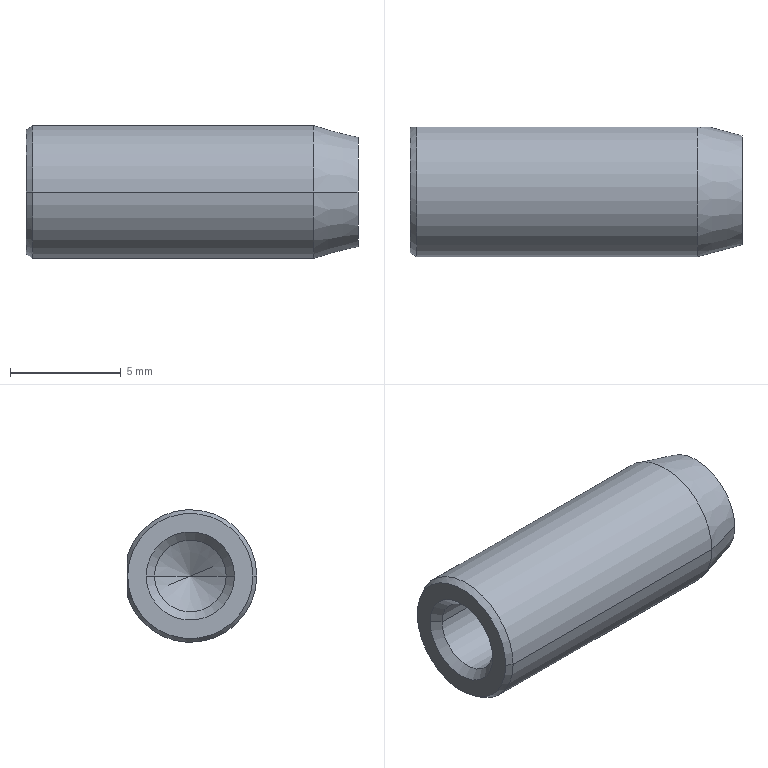Part | STEP file | MSTMS6-15-8 | 1 solid | 15 faces | box 15 x 5.85 x 6 mm | volume 330.192 mm3 | cone 8 | cylinder 4 | plane 3 | commonest cylinder face diameters 3.242 x2 6 x2
STEP:
#1=CARTESIAN_POINT('',(0.,0.,0.));
#2=DIRECTION('',(0.,0.,1.));
#3=DIRECTION('',(1.,0.,0.));
#4=AXIS2_PLACEMENT_3D('',#1,#2,#3);
#5=CARTESIAN_POINT('',(9.464,1.621,0.));
#6=VERTEX_POINT('',#5);
#7=CARTESIAN_POINT('',(9.464,-1.621,0.));
#8=VERTEX_POINT('',#7);
#9=CARTESIAN_POINT('',(9.464,0.,0.));
#10=DIRECTION('',(1.,0.,0.));
#11=DIRECTION('',(0.,-1.,0.));
#12=AXIS2_PLACEMENT_3D('',#9,#10,#11);
#13=CIRCLE('',#12,1.621);
#14=CARTESIAN_POINT('',(9.464,0.,0.));
#15=DIRECTION('',(-1.,0.,0.));
#16=DIRECTION('',(0.,1.,0.));
#17=AXIS2_PLACEMENT_3D('',#14,#15,#16);
#18=CONICAL_SURFACE('',#17,1.621,1.047);
#19=CARTESIAN_POINT('',(9.425,0.));
#20=DIRECTION('',(-1.,0.));
#21=VECTOR('',#20,1.);
#22=LINE('',#19,#21);
#23=(GEOMETRIC_REPRESENTATION_CONTEXT(2)PARAMETRIC_REPRESENTATION_CONTEXT()REPRESENTATION_CONTEXT('',''));
#24=DEFINITIONAL_REPRESENTATION('',(#22),#23);
#25=PCURVE('',#18,#24);
#26=CARTESIAN_POINT('',(10.4,0.,0.));
#27=DIRECTION('',(1.,0.,0.));
#28=DIRECTION('',(0.,-1.,0.));
#29=AXIS2_PLACEMENT_3D('',#26,#27,#28);
#30=CYLINDRICAL_SURFACE('',#29,1.621);
#31=CARTESIAN_POINT('',(0.,-0.9359));
#32=DIRECTION('',(1.,0.));
#33=VECTOR('',#32,1.);
#34=LINE('',#31,#33);
#35=(GEOMETRIC_REPRESENTATION_CONTEXT(2)PARAMETRIC_REPRESENTATION_CONTEXT()REPRESENTATION_CONTEXT('',''));
#36=DEFINITIONAL_REPRESENTATION('',(#34),#35);
#37=PCURVE('',#30,#36);
#38=SURFACE_CURVE('',#13,(#25,#37),.PCURVE_S1.);
#39=EDGE_CURVE('',#6,#8,#38,.T.);
#40=ORIENTED_EDGE('',*,*,#39,.T.);
#41=CARTESIAN_POINT('',(10.4,0.,0.));
#42=VERTEX_POINT('',#41);
#43=CARTESIAN_POINT('',(9.464,-1.621,0.));
#44=DIRECTION('',(-0.5,-0.866,0.));
#45=VECTOR('',#44,1.);
#46=LINE('',#43,#45);
#47=CARTESIAN_POINT('',(3.142,0.));
#48=DIRECTION('',(0.,1.));
#49=VECTOR('',#48,1.);
#50=LINE('',#47,#49);
#51=(GEOMETRIC_REPRESENTATION_CONTEXT(2)PARAMETRIC_REPRESENTATION_CONTEXT()REPRESENTATION_CONTEXT('',''));
#52=DEFINITIONAL_REPRESENTATION('',(#50),#51);
#53=PCURVE('',#18,#52);
#54=CARTESIAN_POINT('',(9.464,0.,0.));
#55=DIRECTION('',(-1.,0.,0.));
#56=DIRECTION('',(0.,1.,0.));
#57=AXIS2_PLACEMENT_3D('',#54,#55,#56);
#58=CONICAL_SURFACE('',#57,1.621,1.047);
#59=CARTESIAN_POINT('',(3.142,0.));
#60=DIRECTION('',(0.,1.));
#61=VECTOR('',#60,1.);
#62=LINE('',#59,#61);
#63=(GEOMETRIC_REPRESENTATION_CONTEXT(2)PARAMETRIC_REPRESENTATION_CONTEXT()REPRESENTATION_CONTEXT('',''));
#64=DEFINITIONAL_REPRESENTATION('',(#62),#63);
#65=PCURVE('',#58,#64);
#66=SURFACE_CURVE('',#46,(#53,#65),.PCURVE_S1.);
#67=EDGE_CURVE('',#42,#8,#66,.T.);
#68=ORIENTED_EDGE('',*,*,#67,.F.);
#69=CARTESIAN_POINT('',(9.464,1.621,0.));
#70=DIRECTION('',(-0.5,0.866,0.));
#71=VECTOR('',#70,1.);
#72=LINE('',#69,#71);
#73=CARTESIAN_POINT('',(6.283,0.));
#74=DIRECTION('',(0.,1.));
#75=VECTOR('',#74,1.);
#76=LINE('',#73,#75);
#77=(GEOMETRIC_REPRESENTATION_CONTEXT(2)PARAMETRIC_REPRESENTATION_CONTEXT()REPRESENTATION_CONTEXT('',''));
#78=DEFINITIONAL_REPRESENTATION('',(#76),#77);
#79=PCURVE('',#18,#78);
#80=CARTESIAN_POINT('',(0.,0.));
#81=DIRECTION('',(0.,1.));
#82=VECTOR('',#81,1.);
#83=LINE('',#80,#82);
#84=(GEOMETRIC_REPRESENTATION_CONTEXT(2)PARAMETRIC_REPRESENTATION_CONTEXT()REPRESENTATION_CONTEXT('',''));
#85=DEFINITIONAL_REPRESENTATION('',(#83),#84);
#86=PCURVE('',#58,#85);
#87=SURFACE_CURVE('',#72,(#79,#86),.PCURVE_S1.);
#88=EDGE_CURVE('',#42,#6,#87,.T.);
#89=ORIENTED_EDGE('',*,*,#88,.T.);
#90=EDGE_LOOP('',(#40,#68,#89));
#91=FACE_BOUND('',#90,.F.);
#92=ADVANCED_FACE('',(#91),#18,.F.);
#93=CARTESIAN_POINT('',(0.379,-1.621,0.));
#94=VERTEX_POINT('',#93);
#95=CARTESIAN_POINT('',(10.4,-1.621,0.));
#96=DIRECTION('',(1.,0.,0.));
#97=VECTOR('',#96,1.);
#98=LINE('',#95,#97);
#99=CARTESIAN_POINT('',(6.283,0.));
#100=DIRECTION('',(0.,1.));
#101=VECTOR('',#100,1.);
#102=LINE('',#99,#101);
#103=(GEOMETRIC_REPRESENTATION_CONTEXT(2)PARAMETRIC_REPRESENTATION_CONTEXT()REPRESENTATION_CONTEXT('',''));
#104=DEFINITIONAL_REPRESENTATION('',(#102),#103);
#105=PCURVE('',#30,#104);
#106=CARTESIAN_POINT('',(10.4,0.,0.));
#107=DIRECTION('',(1.,0.,0.));
#108=DIRECTION('',(0.,-1.,0.));
#109=AXIS2_PLACEMENT_3D('',#106,#107,#108);
#110=CYLINDRICAL_SURFACE('',#109,1.621);
#111=CARTESIAN_POINT('',(0.,0.));
#112=DIRECTION('',(0.,1.));
#113=VECTOR('',#112,1.);
#114=LINE('',#111,#113);
#115=(GEOMETRIC_REPRESENTATION_CONTEXT(2)PARAMETRIC_REPRESENTATION_CONTEXT()REPRESENTATION_CONTEXT('',''));
#116=DEFINITIONAL_REPRESENTATION('',(#114),#115);
#117=PCURVE('',#110,#116);
#118=SURFACE_CURVE('',#98,(#105,#117),.PCURVE_S1.);
#119=EDGE_CURVE('',#94,#8,#118,.T.);
#120=ORIENTED_EDGE('',*,*,#119,.T.);
#121=ORIENTED_EDGE('',*,*,#39,.F.);
#122=CARTESIAN_POINT('',(0.379,1.621,0.));
#123=VERTEX_POINT('',#122);
#124=CARTESIAN_POINT('',(10.4,1.621,0.));
#125=DIRECTION('',(1.,0.,0.));
#126=VECTOR('',#125,1.);
#127=LINE('',#124,#126);
#128=CARTESIAN_POINT('',(3.142,0.));
#129=DIRECTION('',(0.,1.));
#130=VECTOR('',#129,1.);
#131=LINE('',#128,#130);
#132=(GEOMETRIC_REPRESENTATION_CONTEXT(2)PARAMETRIC_REPRESENTATION_CONTEXT()REPRESENTATION_CONTEXT('',''));
#133=DEFINITIONAL_REPRESENTATION('',(#131),#132);
#134=PCURVE('',#30,#133);
#135=CARTESIAN_POINT('',(3.142,0.));
#136=DIRECTION('',(0.,1.));
#137=VECTOR('',#136,1.);
#138=LINE('',#135,#137);
#139=(GEOMETRIC_REPRESENTATION_CONTEXT(2)PARAMETRIC_REPRESENTATION_CONTEXT()REPRESENTATION_CONTEXT('',''));
#140=DEFINITIONAL_REPRESENTATION('',(#138),#139);
#141=PCURVE('',#110,#140);
#142=SURFACE_CURVE('',#127,(#134,#141),.PCURVE_S1.);
#143=EDGE_CURVE('',#123,#6,#142,.T.);
#144=ORIENTED_EDGE('',*,*,#143,.F.);
#145=CARTESIAN_POINT('',(0.379,0.,0.));
#146=DIRECTION('',(1.,0.,0.));
#147=DIRECTION('',(0.,-1.,0.));
#148=AXIS2_PLACEMENT_3D('',#145,#146,#147);
#149=CIRCLE('',#148,1.621);
#150=CARTESIAN_POINT('',(0.,-10.021));
#151=DIRECTION('',(1.,0.));
#152=VECTOR('',#151,1.);
#153=LINE('',#150,#152);
#154=(GEOMETRIC_REPRESENTATION_CONTEXT(2)PARAMETRIC_REPRESENTATION_CONTEXT()REPRESENTATION_CONTEXT('',''));
#155=DEFINITIONAL_REPRESENTATION('',(#153),#154);
#156=PCURVE('',#30,#155);
#157=CARTESIAN_POINT('',(0.,0.,0.));
#158=DIRECTION('',(-1.,0.,0.));
#159=DIRECTION('',(0.,1.,0.));
#160=AXIS2_PLACEMENT_3D('',#157,#158,#159);
#161=CONICAL_SURFACE('',#160,2.,0.7854);
#162=CARTESIAN_POINT('',(9.425,-0.379));
#163=DIRECTION('',(-1.,0.));
#164=VECTOR('',#163,1.);
#165=LINE('',#162,#164);
#166=(GEOMETRIC_REPRESENTATION_CONTEXT(2)PARAMETRIC_REPRESENTATION_CONTEXT()REPRESENTATION_CONTEXT('',''));
#167=DEFINITIONAL_REPRESENTATION('',(#165),#166);
#168=PCURVE('',#161,#167);
#169=SURFACE_CURVE('',#149,(#156,#168),.PCURVE_S1.);
#170=EDGE_CURVE('',#123,#94,#169,.T.);
#171=ORIENTED_EDGE('',*,*,#170,.T.);
#172=EDGE_LOOP('',(#120,#121,#144,#171));
#173=FACE_BOUND('',#172,.F.);
#174=ADVANCED_FACE('',(#173),#30,.F.);
#175=CARTESIAN_POINT('',(0.,2.,0.));
#176=VERTEX_POINT('',#175);
#177=CARTESIAN_POINT('',(0.,2.,0.));
#178=DIRECTION('',(-0.7071,0.7071,0.));
#179=VECTOR('',#178,1.);
#180=LINE('',#177,#179);
#181=CARTESIAN_POINT('',(6.283,0.));
#182=DIRECTION('',(0.,1.));
#183=VECTOR('',#182,1.);
#184=LINE('',#181,#183);
#185=(GEOMETRIC_REPRESENTATION_CONTEXT(2)PARAMETRIC_REPRESENTATION_CONTEXT()REPRESENTATION_CONTEXT('',''));
#186=DEFINITIONAL_REPRESENTATION('',(#184),#185);
#187=PCURVE('',#161,#186);
#188=CARTESIAN_POINT('',(0.,0.,0.));
#189=DIRECTION('',(-1.,0.,0.));
#190=DIRECTION('',(0.,1.,0.));
#191=AXIS2_PLACEMENT_3D('',#188,#189,#190);
#192=CONICAL_SURFACE('',#191,2.,0.7854);
#193=CARTESIAN_POINT('',(0.,0.));
#194=DIRECTION('',(0.,1.));
#195=VECTOR('',#194,1.);
#196=LINE('',#193,#195);
#197=(GEOMETRIC_REPRESENTATION_CONTEXT(2)PARAMETRIC_REPRESENTATION_CONTEXT()REPRESENTATION_CONTEXT('',''));
#198=DEFINITIONAL_REPRESENTATION('',(#196),#197);
#199=PCURVE('',#192,#198);
#200=SURFACE_CURVE('',#180,(#187,#199),.PCURVE_S1.);
#201=EDGE_CURVE('',#123,#176,#200,.T.);
#202=ORIENTED_EDGE('',*,*,#201,.T.);
#203=CARTESIAN_POINT('',(0.,-2.,0.));
#204=VERTEX_POINT('',#203);
#205=CARTESIAN_POINT('',(0.,0.,0.));
#206=DIRECTION('',(1.,0.,0.));
#207=DIRECTION('',(0.,-1.,0.));
#208=AXIS2_PLACEMENT_3D('',#205,#206,#207);
#209=CIRCLE('',#208,2.);
#210=CARTESIAN_POINT('',(9.425,0.));
#211=DIRECTION('',(-1.,0.));
#212=VECTOR('',#211,1.);
#213=LINE('',#210,#212);
#214=(GEOMETRIC_REPRESENTATION_CONTEXT(2)PARAMETRIC_REPRESENTATION_CONTEXT()REPRESENTATION_CONTEXT('',''));
#215=DEFINITIONAL_REPRESENTATION('',(#213),#214);
#216=PCURVE('',#161,#215);
#217=CARTESIAN_POINT('',(0.,0.,0.));
#218=DIRECTION('',(1.,0.,0.));
#219=DIRECTION('',(0.,-1.,0.));
#220=AXIS2_PLACEMENT_3D('',#217,#218,#219);
#221=PLANE('',#220);
#222=CARTESIAN_POINT('',(0.,0.));
#223=DIRECTION('',(1.,0.));
#224=AXIS2_PLACEMENT_2D('',#222,#223);
#225=CIRCLE('',#224,2.);
#226=(GEOMETRIC_REPRESENTATION_CONTEXT(2)PARAMETRIC_REPRESENTATION_CONTEXT()REPRESENTATION_CONTEXT('',''));
#227=DEFINITIONAL_REPRESENTATION('',(#225),#226);
#228=PCURVE('',#221,#227);
#229=SURFACE_CURVE('',#209,(#216,#228),.PCURVE_S1.);
#230=EDGE_CURVE('',#176,#204,#229,.T.);
#231=ORIENTED_EDGE('',*,*,#230,.T.);
#232=CARTESIAN_POINT('',(0.,-2.,0.));
#233=DIRECTION('',(-0.7071,-0.7071,0.));
#234=VECTOR('',#233,1.);
#235=LINE('',#232,#234);
#236=CARTESIAN_POINT('',(3.142,0.));
#237=DIRECTION('',(0.,1.));
#238=VECTOR('',#237,1.);
#239=LINE('',#236,#238);
#240=(GEOMETRIC_REPRESENTATION_CONTEXT(2)PARAMETRIC_REPRESENTATION_CONTEXT()REPRESENTATION_CONTEXT('',''));
#241=DEFINITIONAL_REPRESENTATION('',(#239),#240);
#242=PCURVE('',#161,#241);
#243=CARTESIAN_POINT('',(3.142,0.));
#244=DIRECTION('',(0.,1.));
#245=VECTOR('',#244,1.);
#246=LINE('',#243,#245);
#247=(GEOMETRIC_REPRESENTATION_CONTEXT(2)PARAMETRIC_REPRESENTATION_CONTEXT()REPRESENTATION_CONTEXT('',''));
#248=DEFINITIONAL_REPRESENTATION('',(#246),#247);
#249=PCURVE('',#192,#248);
#250=SURFACE_CURVE('',#235,(#242,#249),.PCURVE_S1.);
#251=EDGE_CURVE('',#94,#204,#250,.T.);
#252=ORIENTED_EDGE('',*,*,#251,.F.);
#253=ORIENTED_EDGE('',*,*,#170,.F.);
#254=EDGE_LOOP('',(#202,#231,#252,#253));
#255=FACE_BOUND('',#254,.F.);
#256=ADVANCED_FACE('',(#255),#161,.F.);
#257=CARTESIAN_POINT('',(15.,-2.464,0.));
#258=VERTEX_POINT('',#257);
#259=CARTESIAN_POINT('',(15.,2.464,0.));
#260=VERTEX_POINT('',#259);
#261=CARTESIAN_POINT('',(15.,0.,0.));
#262=DIRECTION('',(1.,0.,0.));
#263=DIRECTION('',(0.,-1.,0.));
#264=AXIS2_PLACEMENT_3D('',#261,#262,#263);
#265=CIRCLE('',#264,2.464);
#266=CARTESIAN_POINT('',(13.,0.,0.));
#267=DIRECTION('',(-1.,0.,0.));
#268=DIRECTION('',(0.,1.,0.));
#269=AXIS2_PLACEMENT_3D('',#266,#267,#268);
#270=CONICAL_SURFACE('',#269,3.,0.2618);
#271=CARTESIAN_POINT('',(3.142,-2.));
#272=DIRECTION('',(-1.,0.));
#273=VECTOR('',#272,1.);
#274=LINE('',#271,#273);
#275=(GEOMETRIC_REPRESENTATION_CONTEXT(2)PARAMETRIC_REPRESENTATION_CONTEXT()REPRESENTATION_CONTEXT('',''));
#276=DEFINITIONAL_REPRESENTATION('',(#274),#275);
#277=PCURVE('',#270,#276);
#278=CARTESIAN_POINT('',(15.,0.,-2.464));
#279=DIRECTION('',(-1.,0.,0.));
#280=DIRECTION('',(0.,1.,0.));
#281=AXIS2_PLACEMENT_3D('',#278,#279,#280);
#282=PLANE('',#281);
#283=CARTESIAN_POINT('',(-2.464,-2.464));
#284=CARTESIAN_POINT('',(-2.464,1.804));
#285=CARTESIAN_POINT('',(1.232,-0.3301));
#286=CARTESIAN_POINT('',(4.928,-2.464));
#287=CARTESIAN_POINT('',(1.232,-4.598));
#288=CARTESIAN_POINT('',(-2.464,-6.732));
#289=CARTESIAN_POINT('',(-2.464,-2.464));
#290=(BOUNDED_CURVE()B_SPLINE_CURVE(2,(#283,#284,#285,#286,#287,#288,#289),.UNSPECIFIED.,.T.,.F.)B_SPLINE_CURVE_WITH_KNOTS((1,2,2,2,2,1),(-2.094,0.,2.094,4.189,6.283,8.378),.UNSPECIFIED.)CURVE()GEOMETRIC_REPRESENTATION_ITEM()RATIONAL_B_SPLINE_CURVE((1.,0.5,1.,0.5,1.,0.5,1.))REPRESENTATION_ITEM(''));
#291=(GEOMETRIC_REPRESENTATION_CONTEXT(2)PARAMETRIC_REPRESENTATION_CONTEXT()REPRESENTATION_CONTEXT('',''));
#292=DEFINITIONAL_REPRESENTATION('',(#290),#291);
#293=PCURVE('',#282,#292);
#294=SURFACE_CURVE('',#265,(#277,#293),.PCURVE_S1.);
#295=EDGE_CURVE('',#258,#260,#294,.T.);
#296=ORIENTED_EDGE('',*,*,#295,.F.);
#297=CARTESIAN_POINT('',(13.,-3.,0.));
#298=VERTEX_POINT('',#297);
#299=CARTESIAN_POINT('',(13.,-3.,0.));
#300=DIRECTION('',(-0.9659,-0.2588,0.));
#301=VECTOR('',#300,1.);
#302=LINE('',#299,#301);
#303=CARTESIAN_POINT('',(3.142,0.));
#304=DIRECTION('',(0.,1.));
#305=VECTOR('',#304,1.);
#306=LINE('',#303,#305);
#307=(GEOMETRIC_REPRESENTATION_CONTEXT(2)PARAMETRIC_REPRESENTATION_CONTEXT()REPRESENTATION_CONTEXT('',''));
#308=DEFINITIONAL_REPRESENTATION('',(#306),#307);
#309=PCURVE('',#270,#308);
#310=CARTESIAN_POINT('',(13.,0.,0.));
#311=DIRECTION('',(-1.,0.,0.));
#312=DIRECTION('',(0.,1.,0.));
#313=AXIS2_PLACEMENT_3D('',#310,#311,#312);
#314=CONICAL_SURFACE('',#313,3.,0.2618);
#315=CARTESIAN_POINT('',(3.142,0.));
#316=DIRECTION('',(0.,1.));
#317=VECTOR('',#316,1.);
#318=LINE('',#315,#317);
#319=(GEOMETRIC_REPRESENTATION_CONTEXT(2)PARAMETRIC_REPRESENTATION_CONTEXT()REPRESENTATION_CONTEXT('',''));
#320=DEFINITIONAL_REPRESENTATION('',(#318),#319);
#321=PCURVE('',#314,#320);
#322=SURFACE_CURVE('',#302,(#309,#321),.PCURVE_S1.);
#323=EDGE_CURVE('',#258,#298,#322,.T.);
#324=ORIENTED_EDGE('',*,*,#323,.T.);
#325=CARTESIAN_POINT('',(13.,2.85,-0.9367));
#326=VERTEX_POINT('',#325);
#327=CARTESIAN_POINT('',(13.,0.,0.));
#328=DIRECTION('',(1.,0.,0.));
#329=DIRECTION('',(0.,-1.,0.));
#330=AXIS2_PLACEMENT_3D('',#327,#328,#329);
#331=CIRCLE('',#330,3.);
#332=CARTESIAN_POINT('',(3.142,0.));
#333=DIRECTION('',(-1.,0.));
#334=VECTOR('',#333,1.);
#335=LINE('',#332,#334);
#336=(GEOMETRIC_REPRESENTATION_CONTEXT(2)PARAMETRIC_REPRESENTATION_CONTEXT()REPRESENTATION_CONTEXT('',''));
#337=DEFINITIONAL_REPRESENTATION('',(#335),#336);
#338=PCURVE('',#270,#337);
#339=CARTESIAN_POINT('',(15.,0.,0.));
#340=DIRECTION('',(1.,0.,0.));
#341=DIRECTION('',(0.,-1.,0.));
#342=AXIS2_PLACEMENT_3D('',#339,#340,#341);
#343=CYLINDRICAL_SURFACE('',#342,3.);
#344=CARTESIAN_POINT('',(0.,-2.));
#345=DIRECTION('',(1.,0.));
#346=VECTOR('',#345,1.);
#347=LINE('',#344,#346);
#348=(GEOMETRIC_REPRESENTATION_CONTEXT(2)PARAMETRIC_REPRESENTATION_CONTEXT()REPRESENTATION_CONTEXT('',''));
#349=DEFINITIONAL_REPRESENTATION('',(#347),#348);
#350=PCURVE('',#343,#349);
#351=SURFACE_CURVE('',#331,(#338,#350),.PCURVE_S1.);
#352=EDGE_CURVE('',#298,#326,#351,.T.);
#353=ORIENTED_EDGE('',*,*,#352,.T.);
#354=CARTESIAN_POINT('',(13.56,2.85,0.));
#355=VERTEX_POINT('',#354);
#356=CARTESIAN_POINT('',(13.56,2.85,0.));
#357=CARTESIAN_POINT('',(13.56,2.85,-0.0942));
#358=CARTESIAN_POINT('',(13.542,2.85,-0.1877));
#359=CARTESIAN_POINT('',(13.478,2.85,-0.365));
#360=CARTESIAN_POINT('',(13.433,2.85,-0.4473));
#361=CARTESIAN_POINT('',(13.275,2.85,-0.682));
#362=CARTESIAN_POINT('',(13.142,2.85,-0.8146));
#363=CARTESIAN_POINT('',(13.,2.85,-0.9367));
#364=B_SPLINE_CURVE_WITH_KNOTS('',3,(#356,#357,#358,#359,#360,#361,#362,#363),.UNSPECIFIED.,.F.,.F.,(4,2,2,4),(0.008062,0.008341,0.00862,0.009177),.UNSPECIFIED.);
#365=CARTESIAN_POINT('',(0.,-0.5598));
#366=CARTESIAN_POINT('',(0.00601,-0.5598));
#367=CARTESIAN_POINT('',(0.01801,-0.5586));
#368=CARTESIAN_POINT('',(0.03591,-0.5534));
#369=CARTESIAN_POINT('',(0.05362,-0.545));
#370=CARTESIAN_POINT('',(0.0711,-0.5333));
#371=CARTESIAN_POINT('',(0.08827,-0.5188));
#372=CARTESIAN_POINT('',(0.1051,-0.5013));
#373=CARTESIAN_POINT('',(0.1214,-0.4814));
#374=CARTESIAN_POINT('',(0.1373,-0.4593));
#375=CARTESIAN_POINT('',(0.1527,-0.435));
#376=CARTESIAN_POINT('',(0.1678,-0.4088));
#377=CARTESIAN_POINT('',(0.1824,-0.3807));
#378=CARTESIAN_POINT('',(0.1967,-0.3511));
#379=CARTESIAN_POINT('',(0.2105,-0.3204));
#380=CARTESIAN_POINT('',(0.2238,-0.2884));
#381=CARTESIAN_POINT('',(0.2368,-0.2554));
#382=CARTESIAN_POINT('',(0.2493,-0.2214));
#383=CARTESIAN_POINT('',(0.2615,-0.1864));
#384=CARTESIAN_POINT('',(0.2733,-0.1506));
#385=CARTESIAN_POINT('',(0.2848,-0.114));
#386=CARTESIAN_POINT('',(0.296,-0.07662));
#387=CARTESIAN_POINT('',(0.3069,-0.03864));
#388=CARTESIAN_POINT('',(0.314,-0.01294));
#389=CARTESIAN_POINT('',(0.3176,0.));
#390=B_SPLINE_CURVE_WITH_KNOTS('',3,(#365,#366,#367,#368,#369,#370,#371,#372,#373,#374,#375,#376,#377,#378,#379,#380,#381,#382,#383,#384,#385,#386,#387,#388,#389),.UNSPECIFIED.,.F.,.F.,(4,1,1,1,1,1,1,1,1,1,1,1,1,1,1,1,1,1,1,1,1,1,4),(0.008062,0.008113,0.008163,0.008214,0.008265,0.008316,0.008366,0.008417,0.008468,0.008518,0.008569,0.00862,0.00867,0.008721,0.008772,0.008822,0.008873,0.008924,0.008974,0.009025,0.009076,0.009126,0.009177),.QUASI_UNIFORM_KNOTS.);
#391=(GEOMETRIC_REPRESENTATION_CONTEXT(2)PARAMETRIC_REPRESENTATION_CONTEXT()REPRESENTATION_CONTEXT('',''));
#392=DEFINITIONAL_REPRESENTATION('',(#390),#391);
#393=PCURVE('',#270,#392);
#394=CARTESIAN_POINT('',(15.,2.85,3.));
#395=DIRECTION('',(0.,1.,0.));
#396=DIRECTION('',(1.,0.,0.));
#397=AXIS2_PLACEMENT_3D('',#394,#395,#396);
#398=PLANE('',#397);
#399=CARTESIAN_POINT('',(-1.44,3.));
#400=CARTESIAN_POINT('',(-1.44,3.094));
#401=CARTESIAN_POINT('',(-1.458,3.188));
#402=CARTESIAN_POINT('',(-1.522,3.365));
#403=CARTESIAN_POINT('',(-1.567,3.447));
#404=CARTESIAN_POINT('',(-1.725,3.682));
#405=CARTESIAN_POINT('',(-1.858,3.815));
#406=CARTESIAN_POINT('',(-2.,3.937));
#407=B_SPLINE_CURVE_WITH_KNOTS('',3,(#399,#400,#401,#402,#403,#404,#405,#406),.UNSPECIFIED.,.F.,.F.,(4,2,2,4),(0.008062,0.008341,0.00862,0.009177),.UNSPECIFIED.);
#408=(GEOMETRIC_REPRESENTATION_CONTEXT(2)PARAMETRIC_REPRESENTATION_CONTEXT()REPRESENTATION_CONTEXT('',''));
#409=DEFINITIONAL_REPRESENTATION('',(#407),#408);
#410=PCURVE('',#398,#409);
#411=SURFACE_CURVE('',#364,(#393,#410),.PCURVE_S1.);
#412=EDGE_CURVE('',#355,#326,#411,.T.);
#413=ORIENTED_EDGE('',*,*,#412,.F.);
#414=CARTESIAN_POINT('',(13.,3.,0.));
#415=DIRECTION('',(-0.9659,0.2588,0.));
#416=VECTOR('',#415,1.);
#417=LINE('',#414,#416);
#418=CARTESIAN_POINT('',(0.,0.));
#419=DIRECTION('',(0.,1.));
#420=VECTOR('',#419,1.);
#421=LINE('',#418,#420);
#422=(GEOMETRIC_REPRESENTATION_CONTEXT(2)PARAMETRIC_REPRESENTATION_CONTEXT()REPRESENTATION_CONTEXT('',''));
#423=DEFINITIONAL_REPRESENTATION('',(#421),#422);
#424=PCURVE('',#270,#423);
#425=CARTESIAN_POINT('',(6.283,0.));
#426=DIRECTION('',(0.,1.));
#427=VECTOR('',#426,1.);
#428=LINE('',#425,#427);
#429=(GEOMETRIC_REPRESENTATION_CONTEXT(2)PARAMETRIC_REPRESENTATION_CONTEXT()REPRESENTATION_CONTEXT('',''));
#430=DEFINITIONAL_REPRESENTATION('',(#428),#429);
#431=PCURVE('',#314,#430);
#432=SURFACE_CURVE('',#417,(#424,#431),.PCURVE_S1.);
#433=EDGE_CURVE('',#260,#355,#432,.T.);
#434=ORIENTED_EDGE('',*,*,#433,.F.);
#435=EDGE_LOOP('',(#296,#324,#353,#413,#434));
#436=FACE_BOUND('',#435,.T.);
#437=ADVANCED_FACE('',(#436),#270,.T.);
#438=CARTESIAN_POINT('',(0.3,2.85,0.9367));
#439=VERTEX_POINT('',#438);
#440=CARTESIAN_POINT('',(0.3,-3.,0.));
#441=VERTEX_POINT('',#440);
#442=CARTESIAN_POINT('',(0.3,0.,0.));
#443=DIRECTION('',(1.,0.,0.));
#444=DIRECTION('',(0.,-1.,0.));
#445=AXIS2_PLACEMENT_3D('',#442,#443,#444);
#446=CIRCLE('',#445,3.);
#447=CARTESIAN_POINT('',(15.,0.,0.));
#448=DIRECTION('',(1.,0.,0.));
#449=DIRECTION('',(0.,-1.,0.));
#450=AXIS2_PLACEMENT_3D('',#447,#448,#449);
#451=CYLINDRICAL_SURFACE('',#450,3.);
#452=CARTESIAN_POINT('',(0.,-14.7));
#453=DIRECTION('',(1.,0.));
#454=VECTOR('',#453,1.);
#455=LINE('',#452,#454);
#456=(GEOMETRIC_REPRESENTATION_CONTEXT(2)PARAMETRIC_REPRESENTATION_CONTEXT()REPRESENTATION_CONTEXT('',''));
#457=DEFINITIONAL_REPRESENTATION('',(#455),#456);
#458=PCURVE('',#451,#457);
#459=CARTESIAN_POINT('',(0.,0.,0.));
#460=DIRECTION('',(1.,0.,0.));
#461=DIRECTION('',(0.,-1.,0.));
#462=AXIS2_PLACEMENT_3D('',#459,#460,#461);
#463=CONICAL_SURFACE('',#462,2.827,0.5236);
#464=CARTESIAN_POINT('',(0.,0.3));
#465=DIRECTION('',(1.,0.));
#466=VECTOR('',#465,1.);
#467=LINE('',#464,#466);
#468=(GEOMETRIC_REPRESENTATION_CONTEXT(2)PARAMETRIC_REPRESENTATION_CONTEXT()REPRESENTATION_CONTEXT('',''));
#469=DEFINITIONAL_REPRESENTATION('',(#467),#468);
#470=PCURVE('',#463,#469);
#471=SURFACE_CURVE('',#446,(#458,#470),.PCURVE_S1.);
#472=EDGE_CURVE('',#439,#441,#471,.T.);
#473=ORIENTED_EDGE('',*,*,#472,.T.);
#474=CARTESIAN_POINT('',(15.,-3.,0.));
#475=DIRECTION('',(1.,0.,0.));
#476=VECTOR('',#475,1.);
#477=LINE('',#474,#476);
#478=CARTESIAN_POINT('',(6.283,0.));
#479=DIRECTION('',(0.,1.));
#480=VECTOR('',#479,1.);
#481=LINE('',#478,#480);
#482=(GEOMETRIC_REPRESENTATION_CONTEXT(2)PARAMETRIC_REPRESENTATION_CONTEXT()REPRESENTATION_CONTEXT('',''));
#483=DEFINITIONAL_REPRESENTATION('',(#481),#482);
#484=PCURVE('',#451,#483);
#485=CARTESIAN_POINT('',(0.,0.));
#486=DIRECTION('',(0.,1.));
#487=VECTOR('',#486,1.);
#488=LINE('',#485,#487);
#489=(GEOMETRIC_REPRESENTATION_CONTEXT(2)PARAMETRIC_REPRESENTATION_CONTEXT()REPRESENTATION_CONTEXT('',''));
#490=DEFINITIONAL_REPRESENTATION('',(#488),#489);
#491=PCURVE('',#343,#490);
#492=SURFACE_CURVE('',#477,(#484,#491),.PCURVE_S1.);
#493=EDGE_CURVE('',#441,#298,#492,.T.);
#494=ORIENTED_EDGE('',*,*,#493,.T.);
#495=CARTESIAN_POINT('',(13.,2.85,0.9367));
#496=VERTEX_POINT('',#495);
#497=CARTESIAN_POINT('',(13.,0.,0.));
#498=DIRECTION('',(1.,0.,0.));
#499=DIRECTION('',(0.,-1.,0.));
#500=AXIS2_PLACEMENT_3D('',#497,#498,#499);
#501=CIRCLE('',#500,3.);
#502=CARTESIAN_POINT('',(0.,-2.));
#503=DIRECTION('',(1.,0.));
#504=VECTOR('',#503,1.);
#505=LINE('',#502,#504);
#506=(GEOMETRIC_REPRESENTATION_CONTEXT(2)PARAMETRIC_REPRESENTATION_CONTEXT()REPRESENTATION_CONTEXT('',''));
#507=DEFINITIONAL_REPRESENTATION('',(#505),#506);
#508=PCURVE('',#451,#507);
#509=CARTESIAN_POINT('',(9.425,0.));
#510=DIRECTION('',(-1.,0.));
#511=VECTOR('',#510,1.);
#512=LINE('',#509,#511);
#513=(GEOMETRIC_REPRESENTATION_CONTEXT(2)PARAMETRIC_REPRESENTATION_CONTEXT()REPRESENTATION_CONTEXT('',''));
#514=DEFINITIONAL_REPRESENTATION('',(#512),#513);
#515=PCURVE('',#314,#514);
#516=SURFACE_CURVE('',#501,(#508,#515),.PCURVE_S1.);
#517=EDGE_CURVE('',#496,#298,#516,.T.);
#518=ORIENTED_EDGE('',*,*,#517,.F.);
#519=CARTESIAN_POINT('',(15.,2.85,0.9367));
#520=DIRECTION('',(1.,0.,0.));
#521=VECTOR('',#520,1.);
#522=LINE('',#519,#521);
#523=CARTESIAN_POINT('',(3.459,0.));
#524=DIRECTION('',(0.,1.));
#525=VECTOR('',#524,1.);
#526=LINE('',#523,#525);
#527=(GEOMETRIC_REPRESENTATION_CONTEXT(2)PARAMETRIC_REPRESENTATION_CONTEXT()REPRESENTATION_CONTEXT('',''));
#528=DEFINITIONAL_REPRESENTATION('',(#526),#527);
#529=PCURVE('',#451,#528);
#530=CARTESIAN_POINT('',(0.,2.063));
#531=DIRECTION('',(1.,0.));
#532=VECTOR('',#531,1.);
#533=LINE('',#530,#532);
#534=(GEOMETRIC_REPRESENTATION_CONTEXT(2)PARAMETRIC_REPRESENTATION_CONTEXT()REPRESENTATION_CONTEXT('',''));
#535=DEFINITIONAL_REPRESENTATION('',(#533),#534);
#536=PCURVE('',#398,#535);
#537=SURFACE_CURVE('',#522,(#529,#536),.PCURVE_S1.);
#538=EDGE_CURVE('',#439,#496,#537,.T.);
#539=ORIENTED_EDGE('',*,*,#538,.F.);
#540=EDGE_LOOP('',(#473,#494,#518,#539));
#541=FACE_BOUND('',#540,.T.);
#542=ADVANCED_FACE('',(#541),#451,.T.);
#543=CARTESIAN_POINT('',(0.,-2.827,0.));
#544=VERTEX_POINT('',#543);
#545=CARTESIAN_POINT('',(0.,2.827,0.));
#546=VERTEX_POINT('',#545);
#547=CARTESIAN_POINT('',(0.,0.,0.));
#548=DIRECTION('',(1.,0.,0.));
#549=DIRECTION('',(0.,-1.,0.));
#550=AXIS2_PLACEMENT_3D('',#547,#548,#549);
#551=CIRCLE('',#550,2.827);
#552=CARTESIAN_POINT('',(0.,0.,0.));
#553=DIRECTION('',(1.,0.,0.));
#554=DIRECTION('',(0.,-1.,0.));
#555=AXIS2_PLACEMENT_3D('',#552,#553,#554);
#556=CONICAL_SURFACE('',#555,2.827,0.5236);
#557=CARTESIAN_POINT('',(0.,0.));
#558=DIRECTION('',(1.,0.));
#559=VECTOR('',#558,1.);
#560=LINE('',#557,#559);
#561=(GEOMETRIC_REPRESENTATION_CONTEXT(2)PARAMETRIC_REPRESENTATION_CONTEXT()REPRESENTATION_CONTEXT('',''));
#562=DEFINITIONAL_REPRESENTATION('',(#560),#561);
#563=PCURVE('',#556,#562);
#564=CARTESIAN_POINT('',(0.,0.));
#565=DIRECTION('',(1.,0.));
#566=AXIS2_PLACEMENT_2D('',#564,#565);
#567=CIRCLE('',#566,2.827);
#568=(GEOMETRIC_REPRESENTATION_CONTEXT(2)PARAMETRIC_REPRESENTATION_CONTEXT()REPRESENTATION_CONTEXT('',''));
#569=DEFINITIONAL_REPRESENTATION('',(#567),#568);
#570=PCURVE('',#221,#569);
#571=SURFACE_CURVE('',#551,(#563,#570),.PCURVE_S1.);
#572=EDGE_CURVE('',#544,#546,#571,.T.);
#573=ORIENTED_EDGE('',*,*,#572,.T.);
#574=CARTESIAN_POINT('',(0.04019,2.85,0.));
#575=VERTEX_POINT('',#574);
#576=CARTESIAN_POINT('',(0.,2.827,0.));
#577=DIRECTION('',(0.866,0.5,0.));
#578=VECTOR('',#577,1.);
#579=LINE('',#576,#578);
#580=CARTESIAN_POINT('',(3.142,0.));
#581=DIRECTION('',(0.,1.));
#582=VECTOR('',#581,1.);
#583=LINE('',#580,#582);
#584=(GEOMETRIC_REPRESENTATION_CONTEXT(2)PARAMETRIC_REPRESENTATION_CONTEXT()REPRESENTATION_CONTEXT('',''));
#585=DEFINITIONAL_REPRESENTATION('',(#583),#584);
#586=PCURVE('',#556,#585);
#587=CARTESIAN_POINT('',(3.142,0.));
#588=DIRECTION('',(0.,1.));
#589=VECTOR('',#588,1.);
#590=LINE('',#587,#589);
#591=(GEOMETRIC_REPRESENTATION_CONTEXT(2)PARAMETRIC_REPRESENTATION_CONTEXT()REPRESENTATION_CONTEXT('',''));
#592=DEFINITIONAL_REPRESENTATION('',(#590),#591);
#593=PCURVE('',#463,#592);
#594=SURFACE_CURVE('',#579,(#586,#593),.PCURVE_S1.);
#595=EDGE_CURVE('',#546,#575,#594,.T.);
#596=ORIENTED_EDGE('',*,*,#595,.T.);
#597=CARTESIAN_POINT('',(0.3,2.85,-0.9367));
#598=VERTEX_POINT('',#597);
#599=CARTESIAN_POINT('',(0.3,2.85,-0.9367));
#600=CARTESIAN_POINT('',(0.2227,2.85,-0.7939));
#601=CARTESIAN_POINT('',(0.1566,2.85,-0.6414));
#602=CARTESIAN_POINT('',(0.06548,2.85,-0.3277));
#603=CARTESIAN_POINT('',(0.04019,2.85,-0.1642));
#604=CARTESIAN_POINT('',(0.04019,2.85,0.));
#605=B_SPLINE_CURVE_WITH_KNOTS('',3,(#599,#600,#601,#602,#603,#604),.UNSPECIFIED.,.F.,.F.,(4,2,4),(0.007792,0.008281,0.00877),.UNSPECIFIED.);
#606=CARTESIAN_POINT('',(2.824,0.3));
#607=CARTESIAN_POINT('',(2.828,0.293));
#608=CARTESIAN_POINT('',(2.836,0.2791));
#609=CARTESIAN_POINT('',(2.849,0.2589));
#610=CARTESIAN_POINT('',(2.862,0.2393));
#611=CARTESIAN_POINT('',(2.875,0.2204));
#612=CARTESIAN_POINT('',(2.889,0.2023));
#613=CARTESIAN_POINT('',(2.902,0.1849));
#614=CARTESIAN_POINT('',(2.916,0.1683));
#615=CARTESIAN_POINT('',(2.93,0.1525));
#616=CARTESIAN_POINT('',(2.944,0.1377));
#617=CARTESIAN_POINT('',(2.959,0.1238));
#618=CARTESIAN_POINT('',(2.973,0.1109));
#619=CARTESIAN_POINT('',(2.988,0.09893));
#620=CARTESIAN_POINT('',(3.003,0.08803));
#621=CARTESIAN_POINT('',(3.018,0.07818));
#622=CARTESIAN_POINT('',(3.033,0.06941));
#623=CARTESIAN_POINT('',(3.048,0.06173));
#624=CARTESIAN_POINT('',(3.064,0.05517));
#625=CARTESIAN_POINT('',(3.079,0.04976));
#626=CARTESIAN_POINT('',(3.095,0.04551));
#627=CARTESIAN_POINT('',(3.11,0.04246));
#628=CARTESIAN_POINT('',(3.126,0.04061));
#629=CARTESIAN_POINT('',(3.136,0.04019));
#630=CARTESIAN_POINT('',(3.142,0.04019));
#631=B_SPLINE_CURVE_WITH_KNOTS('',3,(#606,#607,#608,#609,#610,#611,#612,#613,#614,#615,#616,#617,#618,#619,#620,#621,#622,#623,#624,#625,#626,#627,#628,#629,#630),.UNSPECIFIED.,.F.,.F.,(4,1,1,1,1,1,1,1,1,1,1,1,1,1,1,1,1,1,1,1,1,1,4),(0.007792,0.007836,0.00788,0.007925,0.007969,0.008014,0.008058,0.008103,0.008147,0.008192,0.008236,0.008281,0.008325,0.00837,0.008414,0.008459,0.008503,0.008548,0.008592,0.008637,0.008681,0.008726,0.00877),.QUASI_UNIFORM_KNOTS.);
#632=(GEOMETRIC_REPRESENTATION_CONTEXT(2)PARAMETRIC_REPRESENTATION_CONTEXT()REPRESENTATION_CONTEXT('',''));
#633=DEFINITIONAL_REPRESENTATION('',(#631),#632);
#634=PCURVE('',#556,#633);
#635=CARTESIAN_POINT('',(-14.7,3.937));
#636=CARTESIAN_POINT('',(-14.777,3.794));
#637=CARTESIAN_POINT('',(-14.843,3.641));
#638=CARTESIAN_POINT('',(-14.935,3.328));
#639=CARTESIAN_POINT('',(-14.96,3.164));
#640=CARTESIAN_POINT('',(-14.96,3.));
#641=B_SPLINE_CURVE_WITH_KNOTS('',3,(#635,#636,#637,#638,#639,#640),.UNSPECIFIED.,.F.,.F.,(4,2,4),(0.007792,0.008281,0.00877),.UNSPECIFIED.);
#642=(GEOMETRIC_REPRESENTATION_CONTEXT(2)PARAMETRIC_REPRESENTATION_CONTEXT()REPRESENTATION_CONTEXT('',''));
#643=DEFINITIONAL_REPRESENTATION('',(#641),#642);
#644=PCURVE('',#398,#643);
#645=SURFACE_CURVE('',#605,(#634,#644),.PCURVE_S1.);
#646=EDGE_CURVE('',#598,#575,#645,.T.);
#647=ORIENTED_EDGE('',*,*,#646,.F.);
#648=CARTESIAN_POINT('',(0.3,0.,0.));
#649=DIRECTION('',(1.,0.,0.));
#650=DIRECTION('',(0.,-1.,0.));
#651=AXIS2_PLACEMENT_3D('',#648,#649,#650);
#652=CIRCLE('',#651,3.);
#653=CARTESIAN_POINT('',(0.,0.3));
#654=DIRECTION('',(1.,0.));
#655=VECTOR('',#654,1.);
#656=LINE('',#653,#655);
#657=(GEOMETRIC_REPRESENTATION_CONTEXT(2)PARAMETRIC_REPRESENTATION_CONTEXT()REPRESENTATION_CONTEXT('',''));
#658=DEFINITIONAL_REPRESENTATION('',(#656),#657);
#659=PCURVE('',#556,#658);
#660=CARTESIAN_POINT('',(0.,-14.7));
#661=DIRECTION('',(1.,0.));
#662=VECTOR('',#661,1.);
#663=LINE('',#660,#662);
#664=(GEOMETRIC_REPRESENTATION_CONTEXT(2)PARAMETRIC_REPRESENTATION_CONTEXT()REPRESENTATION_CONTEXT('',''));
#665=DEFINITIONAL_REPRESENTATION('',(#663),#664);
#666=PCURVE('',#343,#665);
#667=SURFACE_CURVE('',#652,(#659,#666),.PCURVE_S1.);
#668=EDGE_CURVE('',#441,#598,#667,.T.);
#669=ORIENTED_EDGE('',*,*,#668,.F.);
#670=CARTESIAN_POINT('',(0.,-2.827,0.));
#671=DIRECTION('',(0.866,-0.5,0.));
#672=VECTOR('',#671,1.);
#673=LINE('',#670,#672);
#674=CARTESIAN_POINT('',(0.,0.));
#675=DIRECTION('',(0.,1.));
#676=VECTOR('',#675,1.);
#677=LINE('',#674,#676);
#678=(GEOMETRIC_REPRESENTATION_CONTEXT(2)PARAMETRIC_REPRESENTATION_CONTEXT()REPRESENTATION_CONTEXT('',''));
#679=DEFINITIONAL_REPRESENTATION('',(#677),#678);
#680=PCURVE('',#556,#679);
#681=CARTESIAN_POINT('',(6.283,0.));
#682=DIRECTION('',(0.,1.));
#683=VECTOR('',#682,1.);
#684=LINE('',#681,#683);
#685=(GEOMETRIC_REPRESENTATION_CONTEXT(2)PARAMETRIC_REPRESENTATION_CONTEXT()REPRESENTATION_CONTEXT('',''));
#686=DEFINITIONAL_REPRESENTATION('',(#684),#685);
#687=PCURVE('',#463,#686);
#688=SURFACE_CURVE('',#673,(#680,#687),.PCURVE_S1.);
#689=EDGE_CURVE('',#544,#441,#688,.T.);
#690=ORIENTED_EDGE('',*,*,#689,.F.);
#691=EDGE_LOOP('',(#573,#596,#647,#669,#690));
#692=FACE_BOUND('',#691,.T.);
#693=ADVANCED_FACE('',(#692),#556,.T.);
#694=ORIENTED_EDGE('',*,*,#595,.F.);
#695=CARTESIAN_POINT('',(0.,0.,0.));
#696=DIRECTION('',(1.,0.,0.));
#697=DIRECTION('',(0.,-1.,0.));
#698=AXIS2_PLACEMENT_3D('',#695,#696,#697);
#699=CIRCLE('',#698,2.827);
#700=CARTESIAN_POINT('',(0.,0.));
#701=DIRECTION('',(1.,0.));
#702=VECTOR('',#701,1.);
#703=LINE('',#700,#702);
#704=(GEOMETRIC_REPRESENTATION_CONTEXT(2)PARAMETRIC_REPRESENTATION_CONTEXT()REPRESENTATION_CONTEXT('',''));
#705=DEFINITIONAL_REPRESENTATION('',(#703),#704);
#706=PCURVE('',#463,#705);
#707=CARTESIAN_POINT('',(0.,0.));
#708=DIRECTION('',(1.,0.));
#709=AXIS2_PLACEMENT_2D('',#707,#708);
#710=CIRCLE('',#709,2.827);
#711=(GEOMETRIC_REPRESENTATION_CONTEXT(2)PARAMETRIC_REPRESENTATION_CONTEXT()REPRESENTATION_CONTEXT('',''));
#712=DEFINITIONAL_REPRESENTATION('',(#710),#711);
#713=PCURVE('',#221,#712);
#714=SURFACE_CURVE('',#699,(#706,#713),.PCURVE_S1.);
#715=EDGE_CURVE('',#546,#544,#714,.T.);
#716=ORIENTED_EDGE('',*,*,#715,.T.);
#717=ORIENTED_EDGE('',*,*,#689,.T.);
#718=ORIENTED_EDGE('',*,*,#472,.F.);
#719=CARTESIAN_POINT('',(0.04019,2.85,0.));
#720=CARTESIAN_POINT('',(0.04019,2.85,0.1646));
#721=CARTESIAN_POINT('',(0.06497,2.85,0.3258));
#722=CARTESIAN_POINT('',(0.1569,2.85,0.6426));
#723=CARTESIAN_POINT('',(0.2224,2.85,0.7933));
#724=CARTESIAN_POINT('',(0.3,2.85,0.9367));
#725=B_SPLINE_CURVE_WITH_KNOTS('',3,(#719,#720,#721,#722,#723,#724),.UNSPECIFIED.,.F.,.F.,(4,2,4),(0.00877,0.009261,0.009751),.UNSPECIFIED.);
#726=CARTESIAN_POINT('',(3.142,0.04019));
#727=CARTESIAN_POINT('',(3.147,0.04019));
#728=CARTESIAN_POINT('',(3.157,0.0406));
#729=CARTESIAN_POINT('',(3.173,0.04243));
#730=CARTESIAN_POINT('',(3.189,0.04545));
#731=CARTESIAN_POINT('',(3.204,0.04965));
#732=CARTESIAN_POINT('',(3.219,0.05502));
#733=CARTESIAN_POINT('',(3.235,0.06153));
#734=CARTESIAN_POINT('',(3.25,0.06918));
#735=CARTESIAN_POINT('',(3.265,0.07794));
#736=CARTESIAN_POINT('',(3.28,0.0878));
#737=CARTESIAN_POINT('',(3.295,0.09875));
#738=CARTESIAN_POINT('',(3.31,0.1108));
#739=CARTESIAN_POINT('',(3.325,0.1238));
#740=CARTESIAN_POINT('',(3.339,0.1377));
#741=CARTESIAN_POINT('',(3.353,0.1526));
#742=CARTESIAN_POINT('',(3.367,0.1683));
#743=CARTESIAN_POINT('',(3.381,0.1849));
#744=CARTESIAN_POINT('',(3.395,0.2023));
#745=CARTESIAN_POINT('',(3.408,0.2204));
#746=CARTESIAN_POINT('',(3.421,0.2393));
#747=CARTESIAN_POINT('',(3.434,0.2588));
#748=CARTESIAN_POINT('',(3.447,0.279));
#749=CARTESIAN_POINT('',(3.455,0.2929));
#750=CARTESIAN_POINT('',(3.459,0.3));
#751=B_SPLINE_CURVE_WITH_KNOTS('',3,(#726,#727,#728,#729,#730,#731,#732,#733,#734,#735,#736,#737,#738,#739,#740,#741,#742,#743,#744,#745,#746,#747,#748,#749,#750),.UNSPECIFIED.,.F.,.F.,(4,1,1,1,1,1,1,1,1,1,1,1,1,1,1,1,1,1,1,1,1,1,4),(0.00877,0.008815,0.008859,0.008904,0.008949,0.008993,0.009038,0.009082,0.009127,0.009172,0.009216,0.009261,0.009305,0.00935,0.009394,0.009439,0.009484,0.009528,0.009573,0.009617,0.009662,0.009707,0.009751),.QUASI_UNIFORM_KNOTS.);
#752=(GEOMETRIC_REPRESENTATION_CONTEXT(2)PARAMETRIC_REPRESENTATION_CONTEXT()REPRESENTATION_CONTEXT('',''));
#753=DEFINITIONAL_REPRESENTATION('',(#751),#752);
#754=PCURVE('',#463,#753);
#755=CARTESIAN_POINT('',(-14.96,3.));
#756=CARTESIAN_POINT('',(-14.96,2.835));
#757=CARTESIAN_POINT('',(-14.935,2.674));
#758=CARTESIAN_POINT('',(-14.843,2.357));
#759=CARTESIAN_POINT('',(-14.778,2.207));
#760=CARTESIAN_POINT('',(-14.7,2.063));
#761=B_SPLINE_CURVE_WITH_KNOTS('',3,(#755,#756,#757,#758,#759,#760),.UNSPECIFIED.,.F.,.F.,(4,2,4),(0.00877,0.009261,0.009751),.UNSPECIFIED.);
#762=(GEOMETRIC_REPRESENTATION_CONTEXT(2)PARAMETRIC_REPRESENTATION_CONTEXT()REPRESENTATION_CONTEXT('',''));
#763=DEFINITIONAL_REPRESENTATION('',(#761),#762);
#764=PCURVE('',#398,#763);
#765=SURFACE_CURVE('',#725,(#754,#764),.PCURVE_S1.);
#766=EDGE_CURVE('',#575,#439,#765,.T.);
#767=ORIENTED_EDGE('',*,*,#766,.F.);
#768=EDGE_LOOP('',(#694,#716,#717,#718,#767));
#769=FACE_BOUND('',#768,.T.);
#770=ADVANCED_FACE('',(#769),#463,.T.);
#771=ORIENTED_EDGE('',*,*,#493,.F.);
#772=ORIENTED_EDGE('',*,*,#668,.T.);
#773=CARTESIAN_POINT('',(15.,2.85,-0.9367));
#774=DIRECTION('',(-1.,0.,0.));
#775=VECTOR('',#774,1.);
#776=LINE('',#773,#775);
#777=CARTESIAN_POINT('',(2.824,0.));
#778=DIRECTION('',(0.,-1.));
#779=VECTOR('',#778,1.);
#780=LINE('',#777,#779);
#781=(GEOMETRIC_REPRESENTATION_CONTEXT(2)PARAMETRIC_REPRESENTATION_CONTEXT()REPRESENTATION_CONTEXT('',''));
#782=DEFINITIONAL_REPRESENTATION('',(#780),#781);
#783=PCURVE('',#343,#782);
#784=CARTESIAN_POINT('',(0.,3.937));
#785=DIRECTION('',(-1.,0.));
#786=VECTOR('',#785,1.);
#787=LINE('',#784,#786);
#788=(GEOMETRIC_REPRESENTATION_CONTEXT(2)PARAMETRIC_REPRESENTATION_CONTEXT()REPRESENTATION_CONTEXT('',''));
#789=DEFINITIONAL_REPRESENTATION('',(#787),#788);
#790=PCURVE('',#398,#789);
#791=SURFACE_CURVE('',#776,(#783,#790),.PCURVE_S1.);
#792=EDGE_CURVE('',#326,#598,#791,.T.);
#793=ORIENTED_EDGE('',*,*,#792,.F.);
#794=ORIENTED_EDGE('',*,*,#352,.F.);
#795=EDGE_LOOP('',(#771,#772,#793,#794));
#796=FACE_BOUND('',#795,.T.);
#797=ADVANCED_FACE('',(#796),#343,.T.);
#798=ORIENTED_EDGE('',*,*,#323,.F.);
#799=CARTESIAN_POINT('',(15.,0.,0.));
#800=DIRECTION('',(1.,0.,0.));
#801=DIRECTION('',(0.,-1.,0.));
#802=AXIS2_PLACEMENT_3D('',#799,#800,#801);
#803=CIRCLE('',#802,2.464);
#804=CARTESIAN_POINT('',(9.425,-2.));
#805=DIRECTION('',(-1.,0.));
#806=VECTOR('',#805,1.);
#807=LINE('',#804,#806);
#808=(GEOMETRIC_REPRESENTATION_CONTEXT(2)PARAMETRIC_REPRESENTATION_CONTEXT()REPRESENTATION_CONTEXT('',''));
#809=DEFINITIONAL_REPRESENTATION('',(#807),#808);
#810=PCURVE('',#314,#809);
#811=CARTESIAN_POINT('',(-2.464,-2.464));
#812=CARTESIAN_POINT('',(-2.464,1.804));
#813=CARTESIAN_POINT('',(1.232,-0.3301));
#814=CARTESIAN_POINT('',(4.928,-2.464));
#815=CARTESIAN_POINT('',(1.232,-4.598));
#816=CARTESIAN_POINT('',(-2.464,-6.732));
#817=CARTESIAN_POINT('',(-2.464,-2.464));
#818=(BOUNDED_CURVE()B_SPLINE_CURVE(2,(#811,#812,#813,#814,#815,#816,#817),.UNSPECIFIED.,.T.,.F.)B_SPLINE_CURVE_WITH_KNOTS((1,2,2,2,2,1),(-2.094,0.,2.094,4.189,6.283,8.378),.UNSPECIFIED.)CURVE()GEOMETRIC_REPRESENTATION_ITEM()RATIONAL_B_SPLINE_CURVE((1.,0.5,1.,0.5,1.,0.5,1.))REPRESENTATION_ITEM(''));
#819=(GEOMETRIC_REPRESENTATION_CONTEXT(2)PARAMETRIC_REPRESENTATION_CONTEXT()REPRESENTATION_CONTEXT('',''));
#820=DEFINITIONAL_REPRESENTATION('',(#818),#819);
#821=PCURVE('',#282,#820);
#822=SURFACE_CURVE('',#803,(#810,#821),.PCURVE_S1.);
#823=EDGE_CURVE('',#260,#258,#822,.T.);
#824=ORIENTED_EDGE('',*,*,#823,.F.);
#825=ORIENTED_EDGE('',*,*,#433,.T.);
#826=CARTESIAN_POINT('',(13.,2.85,0.9367));
#827=CARTESIAN_POINT('',(13.142,2.85,0.8152));
#828=CARTESIAN_POINT('',(13.275,2.85,0.6804));
#829=CARTESIAN_POINT('',(13.432,2.85,0.4498));
#830=CARTESIAN_POINT('',(13.477,2.85,0.3665));
#831=CARTESIAN_POINT('',(13.542,2.85,0.1886));
#832=CARTESIAN_POINT('',(13.56,2.85,0.09452));
#833=CARTESIAN_POINT('',(13.56,2.85,0.));
#834=B_SPLINE_CURVE_WITH_KNOTS('',3,(#826,#827,#828,#829,#830,#831,#832,#833),.UNSPECIFIED.,.F.,.F.,(4,2,2,4),(0.006943,0.007503,0.007782,0.008062),.UNSPECIFIED.);
#835=CARTESIAN_POINT('',(5.966,0.));
#836=CARTESIAN_POINT('',(5.969,-0.01288));
#837=CARTESIAN_POINT('',(5.976,-0.0385));
#838=CARTESIAN_POINT('',(5.987,-0.07644));
#839=CARTESIAN_POINT('',(5.998,-0.1138));
#840=CARTESIAN_POINT('',(6.01,-0.1505));
#841=CARTESIAN_POINT('',(6.022,-0.1864));
#842=CARTESIAN_POINT('',(6.034,-0.2214));
#843=CARTESIAN_POINT('',(6.047,-0.2555));
#844=CARTESIAN_POINT('',(6.059,-0.2885));
#845=CARTESIAN_POINT('',(6.073,-0.3203));
#846=CARTESIAN_POINT('',(6.086,-0.3508));
#847=CARTESIAN_POINT('',(6.1,-0.38));
#848=CARTESIAN_POINT('',(6.115,-0.4077));
#849=CARTESIAN_POINT('',(6.13,-0.4339));
#850=CARTESIAN_POINT('',(6.145,-0.4583));
#851=CARTESIAN_POINT('',(6.161,-0.4807));
#852=CARTESIAN_POINT('',(6.178,-0.5008));
#853=CARTESIAN_POINT('',(6.195,-0.5184));
#854=CARTESIAN_POINT('',(6.212,-0.5331));
#855=CARTESIAN_POINT('',(6.229,-0.5448));
#856=CARTESIAN_POINT('',(6.247,-0.5534));
#857=CARTESIAN_POINT('',(6.265,-0.5586));
#858=CARTESIAN_POINT('',(6.277,-0.5598));
#859=CARTESIAN_POINT('',(6.283,-0.5598));
#860=B_SPLINE_CURVE_WITH_KNOTS('',3,(#835,#836,#837,#838,#839,#840,#841,#842,#843,#844,#845,#846,#847,#848,#849,#850,#851,#852,#853,#854,#855,#856,#857,#858,#859),.UNSPECIFIED.,.F.,.F.,(4,1,1,1,1,1,1,1,1,1,1,1,1,1,1,1,1,1,1,1,1,1,4),(0.006943,0.006994,0.007045,0.007096,0.007147,0.007198,0.007248,0.007299,0.00735,0.007401,0.007452,0.007503,0.007554,0.007604,0.007655,0.007706,0.007757,0.007808,0.007859,0.00791,0.00796,0.008011,0.008062),.QUASI_UNIFORM_KNOTS.);
#861=(GEOMETRIC_REPRESENTATION_CONTEXT(2)PARAMETRIC_REPRESENTATION_CONTEXT()REPRESENTATION_CONTEXT('',''));
#862=DEFINITIONAL_REPRESENTATION('',(#860),#861);
#863=PCURVE('',#314,#862);
#864=CARTESIAN_POINT('',(-2.,2.063));
#865=CARTESIAN_POINT('',(-1.858,2.185));
#866=CARTESIAN_POINT('',(-1.725,2.32));
#867=CARTESIAN_POINT('',(-1.568,2.55));
#868=CARTESIAN_POINT('',(-1.523,2.633));
#869=CARTESIAN_POINT('',(-1.458,2.811));
#870=CARTESIAN_POINT('',(-1.44,2.905));
#871=CARTESIAN_POINT('',(-1.44,3.));
#872=B_SPLINE_CURVE_WITH_KNOTS('',3,(#864,#865,#866,#867,#868,#869,#870,#871),.UNSPECIFIED.,.F.,.F.,(4,2,2,4),(0.006943,0.007503,0.007782,0.008062),.UNSPECIFIED.);
#873=(GEOMETRIC_REPRESENTATION_CONTEXT(2)PARAMETRIC_REPRESENTATION_CONTEXT()REPRESENTATION_CONTEXT('',''));
#874=DEFINITIONAL_REPRESENTATION('',(#872),#873);
#875=PCURVE('',#398,#874);
#876=SURFACE_CURVE('',#834,(#863,#875),.PCURVE_S1.);
#877=EDGE_CURVE('',#496,#355,#876,.T.);
#878=ORIENTED_EDGE('',*,*,#877,.F.);
#879=ORIENTED_EDGE('',*,*,#517,.T.);
#880=EDGE_LOOP('',(#798,#824,#825,#878,#879));
#881=FACE_BOUND('',#880,.T.);
#882=ADVANCED_FACE('',(#881),#314,.T.);
#883=ORIENTED_EDGE('',*,*,#572,.F.);
#884=ORIENTED_EDGE('',*,*,#715,.F.);
#885=EDGE_LOOP('',(#883,#884));
#886=FACE_BOUND('',#885,.T.);
#887=ORIENTED_EDGE('',*,*,#230,.T.);
#888=CARTESIAN_POINT('',(0.,0.,0.));
#889=DIRECTION('',(1.,0.,0.));
#890=DIRECTION('',(0.,-1.,0.));
#891=AXIS2_PLACEMENT_3D('',#888,#889,#890);
#892=CIRCLE('',#891,2.);
#893=CARTESIAN_POINT('',(0.,0.));
#894=DIRECTION('',(1.,0.));
#895=AXIS2_PLACEMENT_2D('',#893,#894);
#896=CIRCLE('',#895,2.);
#897=(GEOMETRIC_REPRESENTATION_CONTEXT(2)PARAMETRIC_REPRESENTATION_CONTEXT()REPRESENTATION_CONTEXT('',''));
#898=DEFINITIONAL_REPRESENTATION('',(#896),#897);
#899=PCURVE('',#221,#898);
#900=CARTESIAN_POINT('',(3.142,0.));
#901=DIRECTION('',(-1.,0.));
#902=VECTOR('',#901,1.);
#903=LINE('',#900,#902);
#904=(GEOMETRIC_REPRESENTATION_CONTEXT(2)PARAMETRIC_REPRESENTATION_CONTEXT()REPRESENTATION_CONTEXT('',''));
#905=DEFINITIONAL_REPRESENTATION('',(#903),#904);
#906=PCURVE('',#192,#905);
#907=SURFACE_CURVE('',#892,(#899,#906),.PCURVE_S1.);
#908=EDGE_CURVE('',#204,#176,#907,.T.);
#909=ORIENTED_EDGE('',*,*,#908,.T.);
#910=EDGE_LOOP('',(#887,#909));
#911=FACE_BOUND('',#910,.T.);
#912=ADVANCED_FACE('',(#886,#911),#221,.F.);
#913=ORIENTED_EDGE('',*,*,#823,.T.);
#914=ORIENTED_EDGE('',*,*,#295,.T.);
#915=EDGE_LOOP('',(#913,#914));
#916=FACE_BOUND('',#915,.T.);
#917=ADVANCED_FACE('',(#916),#282,.F.);
#918=ORIENTED_EDGE('',*,*,#908,.T.);
#919=ORIENTED_EDGE('',*,*,#201,.F.);
#920=CARTESIAN_POINT('',(0.379,0.,0.));
#921=DIRECTION('',(1.,0.,0.));
#922=DIRECTION('',(0.,-1.,0.));
#923=AXIS2_PLACEMENT_3D('',#920,#921,#922);
#924=CIRCLE('',#923,1.621);
#925=CARTESIAN_POINT('',(3.142,-0.379));
#926=DIRECTION('',(-1.,0.));
#927=VECTOR('',#926,1.);
#928=LINE('',#925,#927);
#929=(GEOMETRIC_REPRESENTATION_CONTEXT(2)PARAMETRIC_REPRESENTATION_CONTEXT()REPRESENTATION_CONTEXT('',''));
#930=DEFINITIONAL_REPRESENTATION('',(#928),#929);
#931=PCURVE('',#192,#930);
#932=CARTESIAN_POINT('',(0.,-10.021));
#933=DIRECTION('',(1.,0.));
#934=VECTOR('',#933,1.);
#935=LINE('',#932,#934);
#936=(GEOMETRIC_REPRESENTATION_CONTEXT(2)PARAMETRIC_REPRESENTATION_CONTEXT()REPRESENTATION_CONTEXT('',''));
#937=DEFINITIONAL_REPRESENTATION('',(#935),#936);
#938=PCURVE('',#110,#937);
#939=SURFACE_CURVE('',#924,(#931,#938),.PCURVE_S1.);
#940=EDGE_CURVE('',#94,#123,#939,.T.);
#941=ORIENTED_EDGE('',*,*,#940,.F.);
#942=ORIENTED_EDGE('',*,*,#251,.T.);
#943=EDGE_LOOP('',(#918,#919,#941,#942));
#944=FACE_BOUND('',#943,.F.);
#945=ADVANCED_FACE('',(#944),#192,.F.);
#946=CARTESIAN_POINT('',(9.464,0.,0.));
#947=DIRECTION('',(1.,0.,0.));
#948=DIRECTION('',(0.,-1.,0.));
#949=AXIS2_PLACEMENT_3D('',#946,#947,#948);
#950=CIRCLE('',#949,1.621);
#951=CARTESIAN_POINT('',(0.,-0.9359));
#952=DIRECTION('',(1.,0.));
#953=VECTOR('',#952,1.);
#954=LINE('',#951,#953);
#955=(GEOMETRIC_REPRESENTATION_CONTEXT(2)PARAMETRIC_REPRESENTATION_CONTEXT()REPRESENTATION_CONTEXT('',''));
#956=DEFINITIONAL_REPRESENTATION('',(#954),#955);
#957=PCURVE('',#110,#956);
#958=CARTESIAN_POINT('',(3.142,0.));
#959=DIRECTION('',(-1.,0.));
#960=VECTOR('',#959,1.);
#961=LINE('',#958,#960);
#962=(GEOMETRIC_REPRESENTATION_CONTEXT(2)PARAMETRIC_REPRESENTATION_CONTEXT()REPRESENTATION_CONTEXT('',''));
#963=DEFINITIONAL_REPRESENTATION('',(#961),#962);
#964=PCURVE('',#58,#963);
#965=SURFACE_CURVE('',#950,(#957,#964),.PCURVE_S1.);
#966=EDGE_CURVE('',#8,#6,#965,.T.);
#967=ORIENTED_EDGE('',*,*,#966,.F.);
#968=ORIENTED_EDGE('',*,*,#119,.F.);
#969=ORIENTED_EDGE('',*,*,#940,.T.);
#970=ORIENTED_EDGE('',*,*,#143,.T.);
#971=EDGE_LOOP('',(#967,#968,#969,#970));
#972=FACE_BOUND('',#971,.F.);
#973=ADVANCED_FACE('',(#972),#110,.F.);
#974=ORIENTED_EDGE('',*,*,#966,.T.);
#975=ORIENTED_EDGE('',*,*,#88,.F.);
#976=ORIENTED_EDGE('',*,*,#67,.T.);
#977=EDGE_LOOP('',(#974,#975,#976));
#978=FACE_BOUND('',#977,.F.);
#979=ADVANCED_FACE('',(#978),#58,.F.);
#980=ORIENTED_EDGE('',*,*,#646,.T.);
#981=ORIENTED_EDGE('',*,*,#766,.T.);
#982=ORIENTED_EDGE('',*,*,#538,.T.);
#983=ORIENTED_EDGE('',*,*,#877,.T.);
#984=ORIENTED_EDGE('',*,*,#412,.T.);
#985=ORIENTED_EDGE('',*,*,#792,.T.);
#986=EDGE_LOOP('',(#980,#981,#982,#983,#984,#985));
#987=FACE_BOUND('',#986,.T.);
#988=ADVANCED_FACE('',(#987),#398,.T.);
#989=CLOSED_SHELL('',(#92,#174,#256,#437,#542,#693,#770,#797,#882,#912,#917,#945,#973,#979,#988));
#990=MANIFOLD_SOLID_BREP('',#989);
#991=(LENGTH_UNIT()NAMED_UNIT(*)SI_UNIT(.MILLI.,.METRE.));
#992=UNCERTAINTY_MEASURE_WITH_UNIT(LENGTH_MEASURE(0.00002),#991,'','');
#993=(NAMED_UNIT(*)PLANE_ANGLE_UNIT()SI_UNIT($,.RADIAN.));
#994=(NAMED_UNIT(*)SI_UNIT($,.STERADIAN.)SOLID_ANGLE_UNIT());
#995=(GEOMETRIC_REPRESENTATION_CONTEXT(3)GLOBAL_UNCERTAINTY_ASSIGNED_CONTEXT((#992))GLOBAL_UNIT_ASSIGNED_CONTEXT((#991,#993,#994))REPRESENTATION_CONTEXT('',''));
#996=ADVANCED_BREP_SHAPE_REPRESENTATION('',(#4,#990),#995);